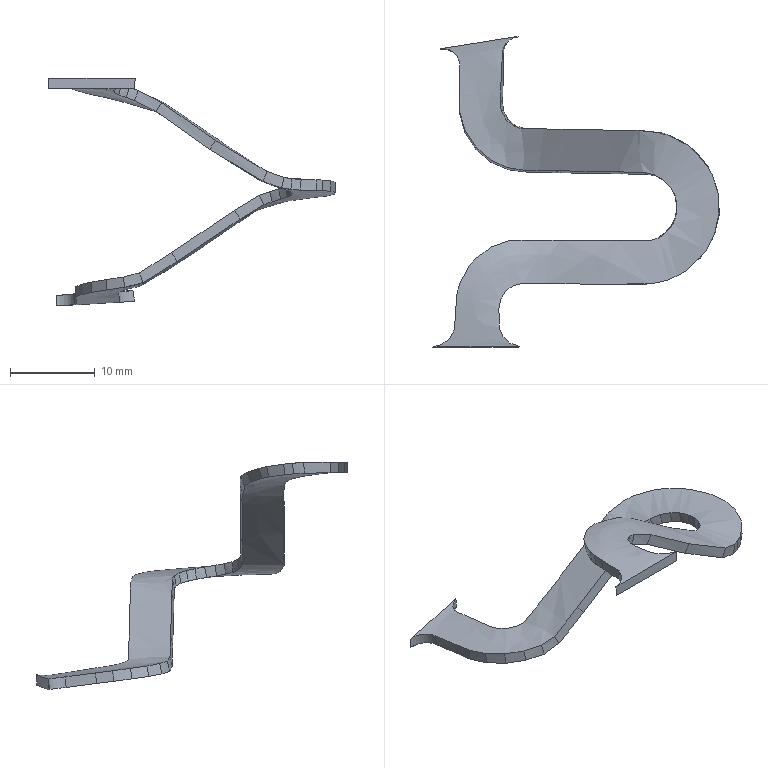Part | STEP file | gslz 2016.10.28-13_id1258_x_t | 1 solid | 75 faces | volume 526.34 mm3 | spline 75